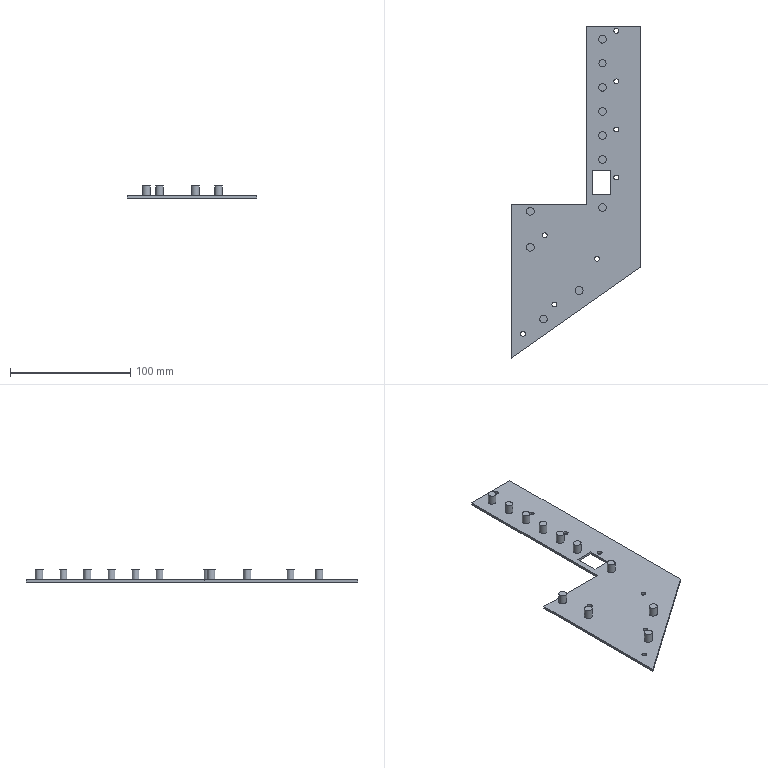Part | STEP file | PCB-R | 1 solid | 42 faces | box 108 x 276 x 10 mm | volume 34872 mm3 | plane 23 | cylinder 19 | commonest cylinder face diameters 6.5 x10 4 x8 5.882 x1